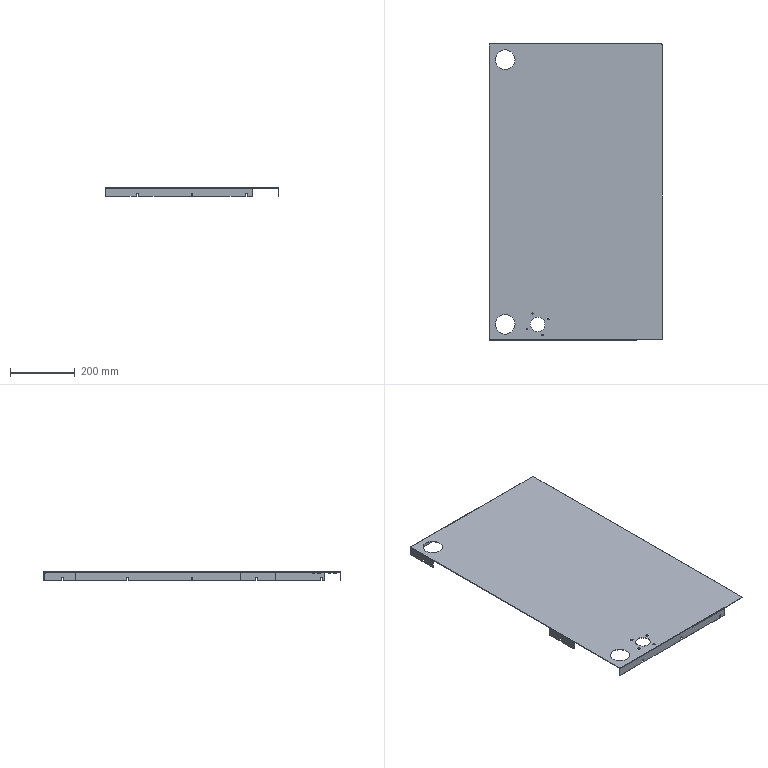Part | STEP file | 1 solid | 174 faces | box 537 x 917 x 27.5 mm | volume 799133 mm3 | plane 89 | cylinder 85 | commonest cylinder face diameters 2 x27 6 x19 4.2 x8 8 x8 4 x7 0.02 x4